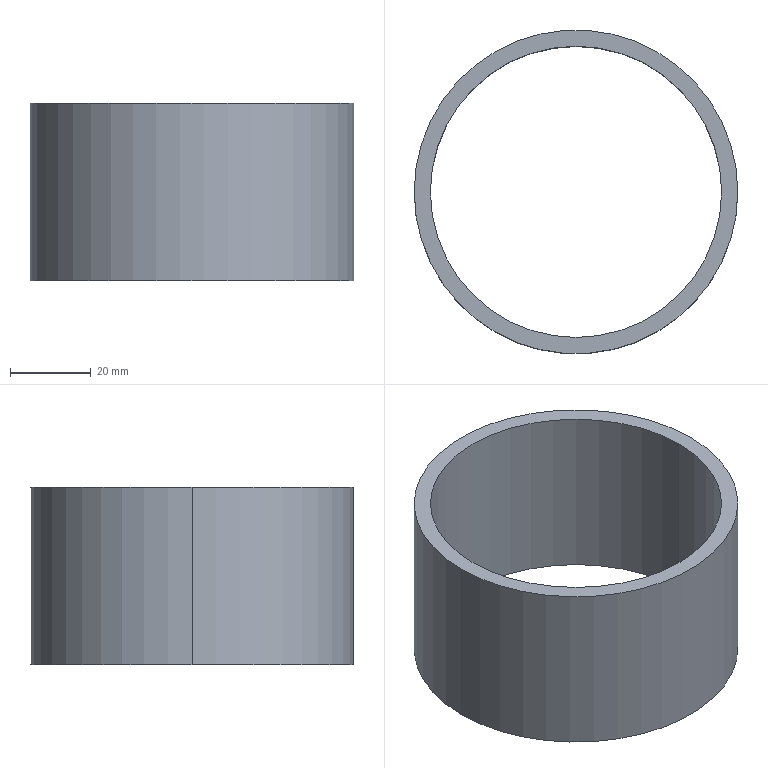Part | SolidWorks | features Extrusion 1 | 1 solid | 6 faces | box 80 x 80 x 44 mm | volume 42022 mm3 | cylinder 4 | plane 2 | commonest cylinder face diameters 72 x2 80 x2
STEP:
#1=CARTESIAN_POINT('',(-1096.,0.,44.));
#2=VERTEX_POINT('',#1);
#3=CARTESIAN_POINT('',(-1024.,0.,44.));
#4=VERTEX_POINT('',#3);
#5=CARTESIAN_POINT('',(-1060.,0.,44.));
#6=DIRECTION('',(0.,0.,1.));
#7=DIRECTION('',(1.,0.,0.));
#8=AXIS2_PLACEMENT_3D('',#5,#6,#7);
#9=CIRCLE('',#8,36.);
#10=EDGE_CURVE('',#2,#4,#9,.T.);
#11=ORIENTED_EDGE('',*,*,#10,.T.);
#12=CARTESIAN_POINT('',(-1024.,0.,0.));
#13=VERTEX_POINT('',#12);
#14=CARTESIAN_POINT('',(-1024.,0.,44.));
#15=DIRECTION('',(0.,0.,-1.));
#16=VECTOR('',#15,1000.);
#17=LINE('',#14,#16);
#18=EDGE_CURVE('',#4,#13,#17,.T.);
#19=ORIENTED_EDGE('',*,*,#18,.T.);
#20=CARTESIAN_POINT('',(-1096.,0.,0.));
#21=VERTEX_POINT('',#20);
#22=CARTESIAN_POINT('',(-1060.,0.,0.));
#23=DIRECTION('',(0.,0.,1.));
#24=DIRECTION('',(1.,0.,0.));
#25=AXIS2_PLACEMENT_3D('',#22,#23,#24);
#26=CIRCLE('',#25,36.);
#27=EDGE_CURVE('',#21,#13,#26,.T.);
#28=ORIENTED_EDGE('',*,*,#27,.F.);
#29=CARTESIAN_POINT('',(-1096.,0.,44.));
#30=DIRECTION('',(0.,0.,-1.));
#31=VECTOR('',#30,1000.);
#32=LINE('',#29,#31);
#33=EDGE_CURVE('',#2,#21,#32,.T.);
#34=ORIENTED_EDGE('',*,*,#33,.F.);
#35=EDGE_LOOP('',(#11,#19,#28,#34));
#36=FACE_OUTER_BOUND('',#35,.T.);
#37=CARTESIAN_POINT('',(-1060.,0.,44.));
#38=DIRECTION('',(0.,0.,-1.));
#39=DIRECTION('',(-1.,0.,0.));
#40=AXIS2_PLACEMENT_3D('',#37,#38,#39);
#41=CYLINDRICAL_SURFACE('',#40,36.);
#42=ADVANCED_FACE('',(#36),#41,.F.);
#43=CARTESIAN_POINT('',(-1020.,0.,44.));
#44=VERTEX_POINT('',#43);
#45=CARTESIAN_POINT('',(-1100.,0.,44.));
#46=VERTEX_POINT('',#45);
#47=CARTESIAN_POINT('',(-1060.,0.,44.));
#48=DIRECTION('',(0.,0.,1.));
#49=DIRECTION('',(1.,0.,0.));
#50=AXIS2_PLACEMENT_3D('',#47,#48,#49);
#51=CIRCLE('',#50,40.);
#52=EDGE_CURVE('',#44,#46,#51,.T.);
#53=ORIENTED_EDGE('',*,*,#52,.F.);
#54=CARTESIAN_POINT('',(-1020.,0.,0.));
#55=VERTEX_POINT('',#54);
#56=CARTESIAN_POINT('',(-1020.,0.,44.));
#57=DIRECTION('',(0.,0.,-1.));
#58=VECTOR('',#57,1000.);
#59=LINE('',#56,#58);
#60=EDGE_CURVE('',#44,#55,#59,.T.);
#61=ORIENTED_EDGE('',*,*,#60,.T.);
#62=CARTESIAN_POINT('',(-1100.,0.,0.));
#63=VERTEX_POINT('',#62);
#64=CARTESIAN_POINT('',(-1060.,0.,0.));
#65=DIRECTION('',(0.,0.,1.));
#66=DIRECTION('',(1.,0.,0.));
#67=AXIS2_PLACEMENT_3D('',#64,#65,#66);
#68=CIRCLE('',#67,40.);
#69=EDGE_CURVE('',#55,#63,#68,.T.);
#70=ORIENTED_EDGE('',*,*,#69,.T.);
#71=CARTESIAN_POINT('',(-1100.,0.,44.));
#72=DIRECTION('',(0.,0.,-1.));
#73=VECTOR('',#72,1000.);
#74=LINE('',#71,#73);
#75=EDGE_CURVE('',#46,#63,#74,.T.);
#76=ORIENTED_EDGE('',*,*,#75,.F.);
#77=EDGE_LOOP('',(#53,#61,#70,#76));
#78=FACE_OUTER_BOUND('',#77,.T.);
#79=CARTESIAN_POINT('',(-1060.,0.,44.));
#80=DIRECTION('',(0.,0.,-1.));
#81=DIRECTION('',(-1.,0.,0.));
#82=AXIS2_PLACEMENT_3D('',#79,#80,#81);
#83=CYLINDRICAL_SURFACE('',#82,40.);
#84=ADVANCED_FACE('',(#78),#83,.T.);
#85=CARTESIAN_POINT('',(-1060.,0.,44.));
#86=DIRECTION('',(0.,0.,1.));
#87=DIRECTION('',(1.,0.,0.));
#88=AXIS2_PLACEMENT_3D('',#85,#86,#87);
#89=CIRCLE('',#88,40.);
#90=EDGE_CURVE('',#46,#44,#89,.T.);
#91=ORIENTED_EDGE('',*,*,#90,.T.);
#92=ORIENTED_EDGE('',*,*,#52,.T.);
#93=EDGE_LOOP('',(#91,#92));
#94=FACE_OUTER_BOUND('',#93,.T.);
#95=ORIENTED_EDGE('',*,*,#10,.F.);
#96=CARTESIAN_POINT('',(-1060.,0.,44.));
#97=DIRECTION('',(0.,0.,1.));
#98=DIRECTION('',(1.,0.,0.));
#99=AXIS2_PLACEMENT_3D('',#96,#97,#98);
#100=CIRCLE('',#99,36.);
#101=EDGE_CURVE('',#4,#2,#100,.T.);
#102=ORIENTED_EDGE('',*,*,#101,.F.);
#103=EDGE_LOOP('',(#95,#102));
#104=FACE_BOUND('',#103,.T.);
#105=CARTESIAN_POINT('',(-1060.,0.,44.));
#106=DIRECTION('',(0.,0.,1.));
#107=DIRECTION('',(1.,0.,0.));
#108=AXIS2_PLACEMENT_3D('',#105,#106,#107);
#109=PLANE('',#108);
#110=ADVANCED_FACE('',(#94,#104),#109,.T.);
#111=CARTESIAN_POINT('',(-1060.,0.,0.));
#112=DIRECTION('',(0.,0.,1.));
#113=DIRECTION('',(1.,0.,0.));
#114=AXIS2_PLACEMENT_3D('',#111,#112,#113);
#115=CIRCLE('',#114,40.);
#116=EDGE_CURVE('',#63,#55,#115,.T.);
#117=ORIENTED_EDGE('',*,*,#116,.F.);
#118=ORIENTED_EDGE('',*,*,#69,.F.);
#119=EDGE_LOOP('',(#117,#118));
#120=FACE_OUTER_BOUND('',#119,.T.);
#121=ORIENTED_EDGE('',*,*,#27,.T.);
#122=CARTESIAN_POINT('',(-1060.,0.,0.));
#123=DIRECTION('',(0.,0.,1.));
#124=DIRECTION('',(1.,0.,0.));
#125=AXIS2_PLACEMENT_3D('',#122,#123,#124);
#126=CIRCLE('',#125,36.);
#127=EDGE_CURVE('',#13,#21,#126,.T.);
#128=ORIENTED_EDGE('',*,*,#127,.T.);
#129=EDGE_LOOP('',(#121,#128));
#130=FACE_BOUND('',#129,.T.);
#131=CARTESIAN_POINT('',(-1060.,0.,0.));
#132=DIRECTION('',(0.,0.,1.));
#133=DIRECTION('',(1.,0.,0.));
#134=AXIS2_PLACEMENT_3D('',#131,#132,#133);
#135=PLANE('',#134);
#136=ADVANCED_FACE('',(#120,#130),#135,.F.);
#137=ORIENTED_EDGE('',*,*,#60,.F.);
#138=ORIENTED_EDGE('',*,*,#90,.F.);
#139=ORIENTED_EDGE('',*,*,#75,.T.);
#140=ORIENTED_EDGE('',*,*,#116,.T.);
#141=EDGE_LOOP('',(#137,#138,#139,#140));
#142=FACE_OUTER_BOUND('',#141,.T.);
#143=CARTESIAN_POINT('',(-1060.,0.,44.));
#144=DIRECTION('',(0.,0.,-1.));
#145=DIRECTION('',(-1.,0.,0.));
#146=AXIS2_PLACEMENT_3D('',#143,#144,#145);
#147=CYLINDRICAL_SURFACE('',#146,40.);
#148=ADVANCED_FACE('',(#142),#147,.T.);
#149=ORIENTED_EDGE('',*,*,#18,.F.);
#150=ORIENTED_EDGE('',*,*,#101,.T.);
#151=ORIENTED_EDGE('',*,*,#33,.T.);
#152=ORIENTED_EDGE('',*,*,#127,.F.);
#153=EDGE_LOOP('',(#149,#150,#151,#152));
#154=FACE_OUTER_BOUND('',#153,.T.);
#155=CARTESIAN_POINT('',(-1060.,0.,44.));
#156=DIRECTION('',(0.,0.,-1.));
#157=DIRECTION('',(-1.,0.,0.));
#158=AXIS2_PLACEMENT_3D('',#155,#156,#157);
#159=CYLINDRICAL_SURFACE('',#158,36.);
#160=ADVANCED_FACE('',(#154),#159,.F.);
#161=CLOSED_SHELL('',(#42,#84,#110,#136,#148,#160));
#162=MANIFOLD_SOLID_BREP('',#161);
#163=CARTESIAN_POINT('',(0.,0.,0.));
#164=DIRECTION('',(0.,0.,1.));
#165=DIRECTION('',(1.,0.,0.));
#166=AXIS2_PLACEMENT_3D('',#163,#164,#165);
#167=(LENGTH_UNIT()NAMED_UNIT(*)SI_UNIT(.MILLI.,.METRE.));
#168=UNCERTAINTY_MEASURE_WITH_UNIT(LENGTH_MEASURE(0.00001),#167,'','');
#169=(NAMED_UNIT(*)PLANE_ANGLE_UNIT()SI_UNIT($,.RADIAN.));
#170=(NAMED_UNIT(*)SI_UNIT($,.STERADIAN.)SOLID_ANGLE_UNIT());
#171=(GEOMETRIC_REPRESENTATION_CONTEXT(3)GLOBAL_UNCERTAINTY_ASSIGNED_CONTEXT((#168))GLOBAL_UNIT_ASSIGNED_CONTEXT((#167,#169,#170))REPRESENTATION_CONTEXT('',''));
#172=ADVANCED_BREP_SHAPE_REPRESENTATION('',(#162,#166),#171);